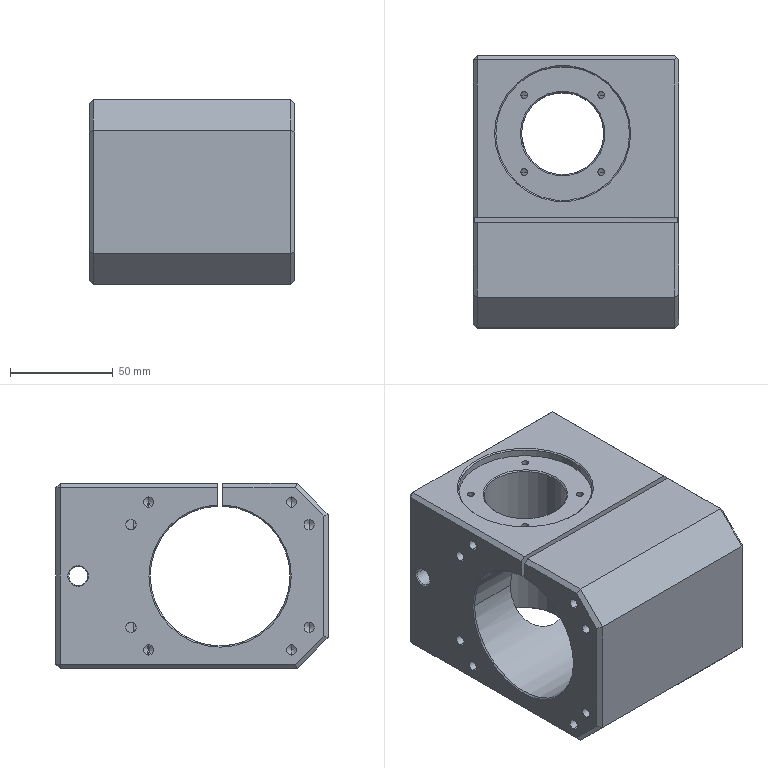Part | SolidWorks | features Chamfer 7, ICE 7, HoleWzd 5, DelFace 4, MoveFace 2, CirPattern 1, Extrusion 1, MirrorPattern 1 | 1 solid | 131 faces | box 100 x 132.3 x 90 mm | volume 668106 mm3 | cylinder 51 | cone 49 | plane 31 | commonest cylinder face diameters 3.3 x16 5 x16 6.8 x8 65 x4 68 x3 9 x2